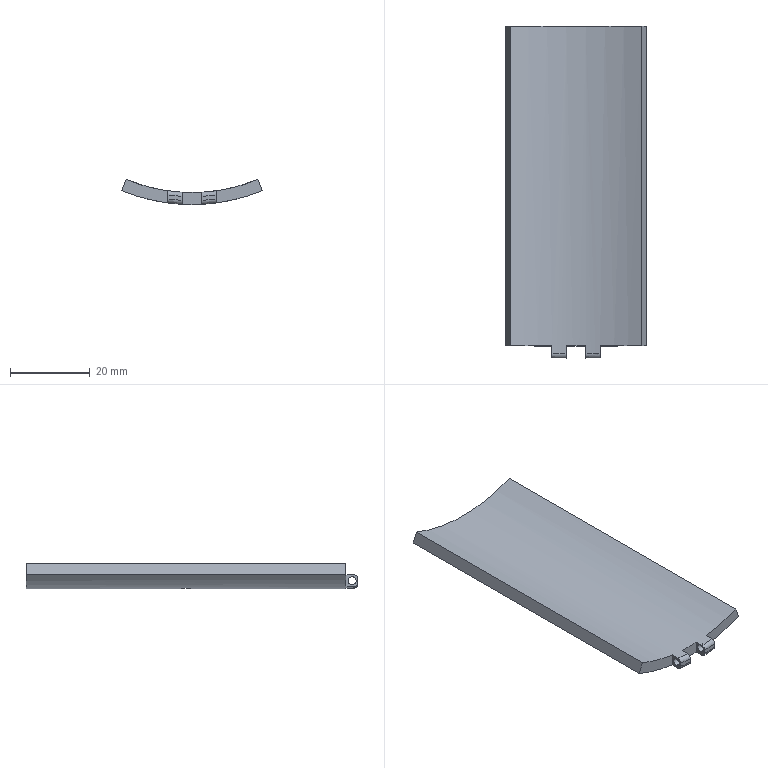Part | SolidWorks | features ICE 3, Blend 1, Fillet 1 | 1 solid | 26 faces | box 35.207 x 83 x 6.273 mm | volume 8409 mm3 | plane 13 | cylinder 9 | torus 4 | commonest cylinder face diameters 2 x4 3 x2 92 x2 86 x1
STEP:
#1=CARTESIAN_POINT('',(-1.5,40.,-45.976));
#2=VERTEX_POINT('',#1);
#3=CARTESIAN_POINT('',(0.,38.5,-46.));
#4=VERTEX_POINT('',#3);
#5=CARTESIAN_POINT('',(-1.5,40.,-45.976));
#6=CARTESIAN_POINT('',(-1.5,39.804,-45.976));
#7=CARTESIAN_POINT('',(-1.461,39.607,-45.977));
#8=CARTESIAN_POINT('',(-1.311,39.246,-45.981));
#9=CARTESIAN_POINT('',(-1.199,39.078,-45.985));
#10=CARTESIAN_POINT('',(-0.9918,38.87,-45.989));
#11=CARTESIAN_POINT('',(-0.9147,38.807,-45.991));
#12=CARTESIAN_POINT('',(-0.7514,38.698,-45.994));
#13=CARTESIAN_POINT('',(-0.6652,38.652,-45.995));
#14=CARTESIAN_POINT('',(-0.4837,38.577,-45.998));
#15=CARTESIAN_POINT('',(-0.3883,38.548,-45.998));
#16=CARTESIAN_POINT('',(-0.1964,38.51,-46.));
#17=CARTESIAN_POINT('',(-0.09898,38.5,-46.));
#18=CARTESIAN_POINT('',(0.,38.5,-46.));
#19=B_SPLINE_CURVE_WITH_KNOTS('',3,(#5,#6,#7,#8,#9,#10,#11,#12,#13,#14,#15,#16,#17,#18),.UNSPECIFIED.,.F.,.F.,(4,2,2,2,2,2,4),(0.00469,0.005276,0.005863,0.006156,0.006449,0.006742,0.007036),.UNSPECIFIED.);
#20=EDGE_CURVE('',#2,#4,#19,.T.);
#21=ORIENTED_EDGE('',*,*,#20,.F.);
#22=CARTESIAN_POINT('',(-1.5,40.,-43.5));
#23=VERTEX_POINT('',#22);
#24=CARTESIAN_POINT('',(-1.5,40.,-46.));
#25=DIRECTION('',(0.,0.,1.));
#26=VECTOR('',#25,1000.);
#27=LINE('',#24,#26);
#28=EDGE_CURVE('',#2,#23,#27,.T.);
#29=ORIENTED_EDGE('',*,*,#28,.T.);
#30=CARTESIAN_POINT('',(1.5,40.,-43.5));
#31=VERTEX_POINT('',#30);
#32=CARTESIAN_POINT('',(0.,40.,-43.5));
#33=DIRECTION('',(0.,0.,1.));
#34=DIRECTION('',(1.,0.,0.));
#35=AXIS2_PLACEMENT_3D('',#32,#33,#34);
#36=CIRCLE('',#35,1.5);
#37=EDGE_CURVE('',#23,#31,#36,.T.);
#38=ORIENTED_EDGE('',*,*,#37,.T.);
#39=CARTESIAN_POINT('',(1.5,40.,-45.976));
#40=VERTEX_POINT('',#39);
#41=CARTESIAN_POINT('',(1.5,40.,-46.));
#42=DIRECTION('',(0.,0.,1.));
#43=VECTOR('',#42,1000.);
#44=LINE('',#41,#43);
#45=EDGE_CURVE('',#40,#31,#44,.T.);
#46=ORIENTED_EDGE('',*,*,#45,.F.);
#47=CARTESIAN_POINT('',(0.,38.5,-46.));
#48=CARTESIAN_POINT('',(0.1978,38.5,-46.));
#49=CARTESIAN_POINT('',(0.3923,38.539,-45.999));
#50=CARTESIAN_POINT('',(0.665,38.652,-45.995));
#51=CARTESIAN_POINT('',(0.7511,38.698,-45.994));
#52=CARTESIAN_POINT('',(0.9139,38.807,-45.991));
#53=CARTESIAN_POINT('',(0.9911,38.87,-45.989));
#54=CARTESIAN_POINT('',(1.199,39.077,-45.985));
#55=CARTESIAN_POINT('',(1.31,39.244,-45.981));
#56=CARTESIAN_POINT('',(1.46,39.605,-45.977));
#57=CARTESIAN_POINT('',(1.5,39.802,-45.976));
#58=CARTESIAN_POINT('',(1.5,40.,-45.976));
#59=B_SPLINE_CURVE_WITH_KNOTS('',3,(#47,#48,#49,#50,#51,#52,#53,#54,#55,#56,#57,#58),.UNSPECIFIED.,.F.,.F.,(4,2,2,2,2,4),(0.007036,0.007622,0.007914,0.008207,0.008793,0.009379),.UNSPECIFIED.);
#60=EDGE_CURVE('',#4,#40,#59,.T.);
#61=ORIENTED_EDGE('',*,*,#60,.F.);
#62=EDGE_LOOP('',(#21,#29,#38,#46,#61));
#63=FACE_OUTER_BOUND('',#62,.T.);
#64=CARTESIAN_POINT('',(0.,40.,-46.));
#65=DIRECTION('',(0.,0.,1.));
#66=DIRECTION('',(1.,0.,0.));
#67=AXIS2_PLACEMENT_3D('',#64,#65,#66);
#68=CYLINDRICAL_SURFACE('',#67,1.5);
#69=ADVANCED_FACE('',(#63),#68,.F.);
#70=CARTESIAN_POINT('',(-6.009,-1.518,-45.081));
#71=VERTEX_POINT('',#70);
#72=CARTESIAN_POINT('',(-6.009,-1.518,-43.081));
#73=VERTEX_POINT('',#72);
#74=CARTESIAN_POINT('',(-6.009,-1.518,-44.081));
#75=DIRECTION('',(-1.,0.,0.));
#76=DIRECTION('',(0.,0.,1.));
#77=AXIS2_PLACEMENT_3D('',#74,#75,#76);
#78=CIRCLE('',#77,1.);
#79=EDGE_CURVE('',#71,#73,#78,.T.);
#80=ORIENTED_EDGE('',*,*,#79,.T.);
#81=CARTESIAN_POINT('',(-2.5,-1.518,-43.081));
#82=VERTEX_POINT('',#81);
#83=CARTESIAN_POINT('',(-6.5,-1.518,-43.081));
#84=DIRECTION('',(1.,0.,0.));
#85=VECTOR('',#84,1000.);
#86=LINE('',#83,#85);
#87=EDGE_CURVE('',#73,#82,#86,.T.);
#88=ORIENTED_EDGE('',*,*,#87,.T.);
#89=CARTESIAN_POINT('',(-2.5,-1.518,-45.081));
#90=VERTEX_POINT('',#89);
#91=CARTESIAN_POINT('',(-2.5,-1.518,-44.081));
#92=DIRECTION('',(1.,0.,0.));
#93=DIRECTION('',(0.,0.,-1.));
#94=AXIS2_PLACEMENT_3D('',#91,#92,#93);
#95=CIRCLE('',#94,1.);
#96=EDGE_CURVE('',#82,#90,#95,.T.);
#97=ORIENTED_EDGE('',*,*,#96,.T.);
#98=CARTESIAN_POINT('',(-6.5,-1.518,-45.081));
#99=DIRECTION('',(1.,0.,0.));
#100=VECTOR('',#99,1000.);
#101=LINE('',#98,#100);
#102=EDGE_CURVE('',#71,#90,#101,.T.);
#103=ORIENTED_EDGE('',*,*,#102,.F.);
#104=EDGE_LOOP('',(#80,#88,#97,#103));
#105=FACE_OUTER_BOUND('',#104,.T.);
#106=CARTESIAN_POINT('',(-6.5,-1.518,-44.081));
#107=DIRECTION('',(1.,0.,0.));
#108=DIRECTION('',(0.,0.,-1.));
#109=AXIS2_PLACEMENT_3D('',#106,#107,#108);
#110=CYLINDRICAL_SURFACE('',#109,1.);
#111=ADVANCED_FACE('',(#105),#110,.F.);
#112=CARTESIAN_POINT('',(2.5,-1.518,-43.081));
#113=VERTEX_POINT('',#112);
#114=CARTESIAN_POINT('',(2.5,-1.518,-45.081));
#115=VERTEX_POINT('',#114);
#116=CARTESIAN_POINT('',(2.5,-1.518,-44.081));
#117=DIRECTION('',(1.,0.,0.));
#118=DIRECTION('',(0.,0.,-1.));
#119=AXIS2_PLACEMENT_3D('',#116,#117,#118);
#120=CIRCLE('',#119,1.);
#121=EDGE_CURVE('',#113,#115,#120,.T.);
#122=ORIENTED_EDGE('',*,*,#121,.F.);
#123=CARTESIAN_POINT('',(6.009,-1.518,-43.081));
#124=VERTEX_POINT('',#123);
#125=CARTESIAN_POINT('',(-6.5,-1.518,-43.081));
#126=DIRECTION('',(1.,0.,0.));
#127=VECTOR('',#126,1000.);
#128=LINE('',#125,#127);
#129=EDGE_CURVE('',#113,#124,#128,.T.);
#130=ORIENTED_EDGE('',*,*,#129,.T.);
#131=CARTESIAN_POINT('',(6.009,-1.518,-45.081));
#132=VERTEX_POINT('',#131);
#133=CARTESIAN_POINT('',(6.009,-1.518,-44.081));
#134=DIRECTION('',(1.,0.,0.));
#135=DIRECTION('',(0.,0.,-1.));
#136=AXIS2_PLACEMENT_3D('',#133,#134,#135);
#137=CIRCLE('',#136,1.);
#138=EDGE_CURVE('',#124,#132,#137,.T.);
#139=ORIENTED_EDGE('',*,*,#138,.T.);
#140=CARTESIAN_POINT('',(-6.5,-1.518,-45.081));
#141=DIRECTION('',(1.,0.,0.));
#142=VECTOR('',#141,1000.);
#143=LINE('',#140,#142);
#144=EDGE_CURVE('',#115,#132,#143,.T.);
#145=ORIENTED_EDGE('',*,*,#144,.F.);
#146=EDGE_LOOP('',(#122,#130,#139,#145));
#147=FACE_OUTER_BOUND('',#146,.T.);
#148=CARTESIAN_POINT('',(-6.5,-1.518,-44.081));
#149=DIRECTION('',(1.,0.,0.));
#150=DIRECTION('',(0.,0.,-1.));
#151=AXIS2_PLACEMENT_3D('',#148,#149,#150);
#152=CYLINDRICAL_SURFACE('',#151,1.);
#153=ADVANCED_FACE('',(#147),#152,.F.);
#154=CARTESIAN_POINT('',(0.,80.,-46.));
#155=VERTEX_POINT('',#154);
#156=CARTESIAN_POINT('',(-17.603,80.,-42.498));
#157=VERTEX_POINT('',#156);
#158=CARTESIAN_POINT('',(0.,80.,0.));
#159=DIRECTION('',(0.,1.,0.));
#160=DIRECTION('',(0.,0.,-1.));
#161=AXIS2_PLACEMENT_3D('',#158,#159,#160);
#162=CIRCLE('',#161,46.);
#163=EDGE_CURVE('',#155,#157,#162,.T.);
#164=ORIENTED_EDGE('',*,*,#163,.F.);
#165=CARTESIAN_POINT('',(0.,41.5,-46.));
#166=VERTEX_POINT('',#165);
#167=CARTESIAN_POINT('',(0.,80.,-46.));
#168=DIRECTION('',(0.,-1.,0.));
#169=VECTOR('',#168,1000.);
#170=LINE('',#167,#169);
#171=EDGE_CURVE('',#155,#166,#170,.T.);
#172=ORIENTED_EDGE('',*,*,#171,.T.);
#173=CARTESIAN_POINT('',(0.,41.5,-46.));
#174=CARTESIAN_POINT('',(-0.09782,41.5,-46.));
#175=CARTESIAN_POINT('',(-0.1972,41.49,-46.));
#176=CARTESIAN_POINT('',(-0.3895,41.452,-45.998));
#177=CARTESIAN_POINT('',(-0.483,41.424,-45.998));
#178=CARTESIAN_POINT('',(-0.6646,41.348,-45.995));
#179=CARTESIAN_POINT('',(-0.7524,41.301,-45.994));
#180=CARTESIAN_POINT('',(-0.9149,41.193,-45.991));
#181=CARTESIAN_POINT('',(-0.9906,41.131,-45.989));
#182=CARTESIAN_POINT('',(-1.201,40.921,-45.985));
#183=CARTESIAN_POINT('',(-1.311,40.756,-45.981));
#184=CARTESIAN_POINT('',(-1.424,40.483,-45.978));
#185=CARTESIAN_POINT('',(-1.452,40.389,-45.977));
#186=CARTESIAN_POINT('',(-1.49,40.197,-45.976));
#187=CARTESIAN_POINT('',(-1.5,40.098,-45.976));
#188=CARTESIAN_POINT('',(-1.5,40.,-45.976));
#189=B_SPLINE_CURVE_WITH_KNOTS('',3,(#173,#174,#175,#176,#177,#178,#179,#180,#181,#182,#183,#184,#185,#186,#187,#188),.UNSPECIFIED.,.F.,.F.,(4,2,2,2,2,2,2,4),(0.002346,0.002639,0.002932,0.003225,0.003518,0.004104,0.004397,0.00469),.UNSPECIFIED.);
#190=EDGE_CURVE('',#166,#2,#189,.T.);
#191=ORIENTED_EDGE('',*,*,#190,.T.);
#192=ORIENTED_EDGE('',*,*,#20,.T.);
#193=CARTESIAN_POINT('',(0.,0.,-46.));
#194=VERTEX_POINT('',#193);
#195=CARTESIAN_POINT('',(0.,80.,-46.));
#196=DIRECTION('',(0.,-1.,0.));
#197=VECTOR('',#196,1000.);
#198=LINE('',#195,#197);
#199=EDGE_CURVE('',#4,#194,#198,.T.);
#200=ORIENTED_EDGE('',*,*,#199,.T.);
#201=CARTESIAN_POINT('',(-2.5,0.,-45.932));
#202=VERTEX_POINT('',#201);
#203=CARTESIAN_POINT('',(0.,0.,0.));
#204=DIRECTION('',(0.,1.,0.));
#205=DIRECTION('',(0.,0.,-1.));
#206=AXIS2_PLACEMENT_3D('',#203,#204,#205);
#207=CIRCLE('',#206,46.);
#208=EDGE_CURVE('',#194,#202,#207,.T.);
#209=ORIENTED_EDGE('',*,*,#208,.T.);
#210=CARTESIAN_POINT('',(-2.5,-2.,-45.932));
#211=VERTEX_POINT('',#210);
#212=CARTESIAN_POINT('',(-2.5,-3.,-45.932));
#213=DIRECTION('',(0.,1.,0.));
#214=VECTOR('',#213,1000.);
#215=LINE('',#212,#214);
#216=EDGE_CURVE('',#211,#202,#215,.T.);
#217=ORIENTED_EDGE('',*,*,#216,.F.);
#218=CARTESIAN_POINT('',(-6.009,-2.,-45.606));
#219=VERTEX_POINT('',#218);
#220=CARTESIAN_POINT('',(0.,-2.,0.));
#221=DIRECTION('',(0.,1.,0.));
#222=DIRECTION('',(0.,0.,-1.));
#223=AXIS2_PLACEMENT_3D('',#220,#221,#222);
#224=CIRCLE('',#223,46.);
#225=EDGE_CURVE('',#211,#219,#224,.T.);
#226=ORIENTED_EDGE('',*,*,#225,.T.);
#227=CARTESIAN_POINT('',(-6.009,0.,-45.606));
#228=VERTEX_POINT('',#227);
#229=CARTESIAN_POINT('',(-6.009,-3.,-45.606));
#230=DIRECTION('',(0.,1.,0.));
#231=VECTOR('',#230,1000.);
#232=LINE('',#229,#231);
#233=EDGE_CURVE('',#219,#228,#232,.T.);
#234=ORIENTED_EDGE('',*,*,#233,.T.);
#235=CARTESIAN_POINT('',(-17.603,0.,-42.498));
#236=VERTEX_POINT('',#235);
#237=CARTESIAN_POINT('',(0.,0.,0.));
#238=DIRECTION('',(0.,1.,0.));
#239=DIRECTION('',(0.,0.,-1.));
#240=AXIS2_PLACEMENT_3D('',#237,#238,#239);
#241=CIRCLE('',#240,46.);
#242=EDGE_CURVE('',#228,#236,#241,.T.);
#243=ORIENTED_EDGE('',*,*,#242,.T.);
#244=CARTESIAN_POINT('',(-17.603,80.,-42.498));
#245=DIRECTION('',(0.,-1.,0.));
#246=VECTOR('',#245,1000.);
#247=LINE('',#244,#246);
#248=EDGE_CURVE('',#157,#236,#247,.T.);
#249=ORIENTED_EDGE('',*,*,#248,.F.);
#250=EDGE_LOOP('',(#164,#172,#191,#192,#200,#209,#217,#226,#234,#243,#249));
#251=FACE_OUTER_BOUND('',#250,.T.);
#252=CARTESIAN_POINT('',(0.,80.,0.));
#253=DIRECTION('',(0.,-1.,0.));
#254=DIRECTION('',(0.,0.,-1.));
#255=AXIS2_PLACEMENT_3D('',#252,#253,#254);
#256=CYLINDRICAL_SURFACE('',#255,46.);
#257=ADVANCED_FACE('',(#251),#256,.T.);
#258=CARTESIAN_POINT('',(2.5,0.,-45.932));
#259=VERTEX_POINT('',#258);
#260=CARTESIAN_POINT('',(0.,0.,0.));
#261=DIRECTION('',(0.,1.,0.));
#262=DIRECTION('',(0.,0.,-1.));
#263=AXIS2_PLACEMENT_3D('',#260,#261,#262);
#264=CIRCLE('',#263,46.);
#265=EDGE_CURVE('',#259,#194,#264,.T.);
#266=ORIENTED_EDGE('',*,*,#265,.F.);
#267=CARTESIAN_POINT('',(2.5,0.,-42.927));
#268=VERTEX_POINT('',#267);
#269=CARTESIAN_POINT('',(2.5,0.,0.));
#270=DIRECTION('',(0.,0.,-1.));
#271=VECTOR('',#270,1000.);
#272=LINE('',#269,#271);
#273=EDGE_CURVE('',#268,#259,#272,.T.);
#274=ORIENTED_EDGE('',*,*,#273,.F.);
#275=CARTESIAN_POINT('',(-2.5,0.,-42.927));
#276=VERTEX_POINT('',#275);
#277=CARTESIAN_POINT('',(0.,0.,0.));
#278=DIRECTION('',(0.,-1.,0.));
#279=DIRECTION('',(0.,0.,-1.));
#280=AXIS2_PLACEMENT_3D('',#277,#278,#279);
#281=CIRCLE('',#280,43.);
#282=EDGE_CURVE('',#276,#268,#281,.T.);
#283=ORIENTED_EDGE('',*,*,#282,.F.);
#284=CARTESIAN_POINT('',(-2.5,0.,0.));
#285=DIRECTION('',(0.,0.,-1.));
#286=VECTOR('',#285,1000.);
#287=LINE('',#284,#286);
#288=EDGE_CURVE('',#276,#202,#287,.T.);
#289=ORIENTED_EDGE('',*,*,#288,.T.);
#290=ORIENTED_EDGE('',*,*,#208,.F.);
#291=EDGE_LOOP('',(#266,#274,#283,#289,#290));
#292=FACE_OUTER_BOUND('',#291,.T.);
#293=CARTESIAN_POINT('',(0.,0.,0.));
#294=DIRECTION('',(0.,-1.,0.));
#295=DIRECTION('',(0.,0.,-1.));
#296=AXIS2_PLACEMENT_3D('',#293,#294,#295);
#297=PLANE('',#296);
#298=ADVANCED_FACE('',(#292),#297,.T.);
#299=ORIENTED_EDGE('',*,*,#242,.F.);
#300=CARTESIAN_POINT('',(-6.009,0.,-42.578));
#301=VERTEX_POINT('',#300);
#302=CARTESIAN_POINT('',(-6.009,0.,0.));
#303=DIRECTION('',(0.,0.,1.));
#304=VECTOR('',#303,1000.);
#305=LINE('',#302,#304);
#306=EDGE_CURVE('',#228,#301,#305,.T.);
#307=ORIENTED_EDGE('',*,*,#306,.T.);
#308=CARTESIAN_POINT('',(-16.455,0.,-39.727));
#309=VERTEX_POINT('',#308);
#310=CARTESIAN_POINT('',(0.,0.,0.));
#311=DIRECTION('',(0.,-1.,0.));
#312=DIRECTION('',(0.,0.,-1.));
#313=AXIS2_PLACEMENT_3D('',#310,#311,#312);
#314=CIRCLE('',#313,43.);
#315=EDGE_CURVE('',#309,#301,#314,.T.);
#316=ORIENTED_EDGE('',*,*,#315,.F.);
#317=CARTESIAN_POINT('',(-17.603,0.,-42.498));
#318=DIRECTION('',(0.3827,0.,0.9239));
#319=VECTOR('',#318,1000.);
#320=LINE('',#317,#319);
#321=EDGE_CURVE('',#236,#309,#320,.T.);
#322=ORIENTED_EDGE('',*,*,#321,.F.);
#323=EDGE_LOOP('',(#299,#307,#316,#322));
#324=FACE_OUTER_BOUND('',#323,.T.);
#325=CARTESIAN_POINT('',(0.,0.,0.));
#326=DIRECTION('',(0.,-1.,0.));
#327=DIRECTION('',(0.,0.,-1.));
#328=AXIS2_PLACEMENT_3D('',#325,#326,#327);
#329=PLANE('',#328);
#330=ADVANCED_FACE('',(#324),#329,.T.);
#331=CARTESIAN_POINT('',(6.009,0.,-42.578));
#332=VERTEX_POINT('',#331);
#333=CARTESIAN_POINT('',(6.009,0.,-45.606));
#334=VERTEX_POINT('',#333);
#335=CARTESIAN_POINT('',(6.009,0.,0.));
#336=DIRECTION('',(0.,0.,-1.));
#337=VECTOR('',#336,1000.);
#338=LINE('',#335,#337);
#339=EDGE_CURVE('',#332,#334,#338,.T.);
#340=ORIENTED_EDGE('',*,*,#339,.T.);
#341=CARTESIAN_POINT('',(17.603,0.,-42.498));
#342=VERTEX_POINT('',#341);
#343=CARTESIAN_POINT('',(0.,0.,0.));
#344=DIRECTION('',(0.,1.,0.));
#345=DIRECTION('',(0.,0.,-1.));
#346=AXIS2_PLACEMENT_3D('',#343,#344,#345);
#347=CIRCLE('',#346,46.);
#348=EDGE_CURVE('',#342,#334,#347,.T.);
#349=ORIENTED_EDGE('',*,*,#348,.F.);
#350=CARTESIAN_POINT('',(16.455,0.,-39.727));
#351=VERTEX_POINT('',#350);
#352=CARTESIAN_POINT('',(17.603,0.,-42.498));
#353=DIRECTION('',(0.3827,0.,-0.9239));
#354=VECTOR('',#353,1000.);
#355=LINE('',#352,#354);
#356=EDGE_CURVE('',#351,#342,#355,.T.);
#357=ORIENTED_EDGE('',*,*,#356,.F.);
#358=CARTESIAN_POINT('',(0.,0.,0.));
#359=DIRECTION('',(0.,-1.,0.));
#360=DIRECTION('',(0.,0.,-1.));
#361=AXIS2_PLACEMENT_3D('',#358,#359,#360);
#362=CIRCLE('',#361,43.);
#363=EDGE_CURVE('',#332,#351,#362,.T.);
#364=ORIENTED_EDGE('',*,*,#363,.F.);
#365=EDGE_LOOP('',(#340,#349,#357,#364));
#366=FACE_OUTER_BOUND('',#365,.T.);
#367=CARTESIAN_POINT('',(0.,0.,0.));
#368=DIRECTION('',(0.,-1.,0.));
#369=DIRECTION('',(0.,0.,-1.));
#370=AXIS2_PLACEMENT_3D('',#367,#368,#369);
#371=PLANE('',#370);
#372=ADVANCED_FACE('',(#366),#371,.T.);
#373=CARTESIAN_POINT('',(-16.455,80.,-39.727));
#374=VERTEX_POINT('',#373);
#375=CARTESIAN_POINT('',(16.455,80.,-39.727));
#376=VERTEX_POINT('',#375);
#377=CARTESIAN_POINT('',(0.,80.,0.));
#378=DIRECTION('',(0.,-1.,0.));
#379=DIRECTION('',(0.,0.,-1.));
#380=AXIS2_PLACEMENT_3D('',#377,#378,#379);
#381=CIRCLE('',#380,43.);
#382=EDGE_CURVE('',#374,#376,#381,.T.);
#383=ORIENTED_EDGE('',*,*,#382,.T.);
#384=CARTESIAN_POINT('',(17.603,80.,-42.498));
#385=VERTEX_POINT('',#384);
#386=CARTESIAN_POINT('',(17.603,80.,-42.498));
#387=DIRECTION('',(0.3827,0.,-0.9239));
#388=VECTOR('',#387,1000.);
#389=LINE('',#386,#388);
#390=EDGE_CURVE('',#376,#385,#389,.T.);
#391=ORIENTED_EDGE('',*,*,#390,.T.);
#392=CARTESIAN_POINT('',(0.,80.,0.));
#393=DIRECTION('',(0.,1.,0.));
#394=DIRECTION('',(0.,0.,-1.));
#395=AXIS2_PLACEMENT_3D('',#392,#393,#394);
#396=CIRCLE('',#395,46.);
#397=EDGE_CURVE('',#385,#155,#396,.T.);
#398=ORIENTED_EDGE('',*,*,#397,.T.);
#399=ORIENTED_EDGE('',*,*,#163,.T.);
#400=CARTESIAN_POINT('',(-17.603,80.,-42.498));
#401=DIRECTION('',(0.3827,0.,0.9239));
#402=VECTOR('',#401,1000.);
#403=LINE('',#400,#402);
#404=EDGE_CURVE('',#157,#374,#403,.T.);
#405=ORIENTED_EDGE('',*,*,#404,.T.);
#406=EDGE_LOOP('',(#383,#391,#398,#399,#405));
#407=FACE_OUTER_BOUND('',#406,.T.);
#408=CARTESIAN_POINT('',(0.,80.,0.));
#409=DIRECTION('',(0.,-1.,0.));
#410=DIRECTION('',(0.,0.,-1.));
#411=AXIS2_PLACEMENT_3D('',#408,#409,#410);
#412=PLANE('',#411);
#413=ADVANCED_FACE('',(#407),#412,.F.);
#414=CARTESIAN_POINT('',(16.455,80.,-39.727));
#415=DIRECTION('',(0.,-1.,0.));
#416=VECTOR('',#415,1000.);
#417=LINE('',#414,#416);
#418=EDGE_CURVE('',#376,#351,#417,.T.);
#419=ORIENTED_EDGE('',*,*,#418,.T.);
#420=ORIENTED_EDGE('',*,*,#356,.T.);
#421=CARTESIAN_POINT('',(17.603,80.,-42.498));
#422=DIRECTION('',(0.,-1.,0.));
#423=VECTOR('',#422,1000.);
#424=LINE('',#421,#423);
#425=EDGE_CURVE('',#385,#342,#424,.T.);
#426=ORIENTED_EDGE('',*,*,#425,.F.);
#427=ORIENTED_EDGE('',*,*,#390,.F.);
#428=EDGE_LOOP('',(#419,#420,#426,#427));
#429=FACE_OUTER_BOUND('',#428,.T.);
#430=CARTESIAN_POINT('',(0.,0.,0.));
#431=DIRECTION('',(0.9239,0.,0.3827));
#432=DIRECTION('',(0.3827,0.,-0.9239));
#433=AXIS2_PLACEMENT_3D('',#430,#431,#432);
#434=PLANE('',#433);
#435=ADVANCED_FACE('',(#429),#434,.T.);
#436=ORIENTED_EDGE('',*,*,#171,.F.);
#437=ORIENTED_EDGE('',*,*,#397,.F.);
#438=ORIENTED_EDGE('',*,*,#425,.T.);
#439=ORIENTED_EDGE('',*,*,#348,.T.);
#440=CARTESIAN_POINT('',(6.009,-2.,-45.606));
#441=VERTEX_POINT('',#440);
#442=CARTESIAN_POINT('',(6.009,-3.,-45.606));
#443=DIRECTION('',(0.,1.,0.));
#444=VECTOR('',#443,1000.);
#445=LINE('',#442,#444);
#446=EDGE_CURVE('',#441,#334,#445,.T.);
#447=ORIENTED_EDGE('',*,*,#446,.F.);
#448=CARTESIAN_POINT('',(2.5,-2.,-45.932));
#449=VERTEX_POINT('',#448);
#450=CARTESIAN_POINT('',(0.,-2.,0.));
#451=DIRECTION('',(0.,1.,0.));
#452=DIRECTION('',(0.,0.,-1.));
#453=AXIS2_PLACEMENT_3D('',#450,#451,#452);
#454=CIRCLE('',#453,46.);
#455=EDGE_CURVE('',#441,#449,#454,.T.);
#456=ORIENTED_EDGE('',*,*,#455,.T.);
#457=CARTESIAN_POINT('',(2.5,-3.,-45.932));
#458=DIRECTION('',(0.,1.,0.));
#459=VECTOR('',#458,1000.);
#460=LINE('',#457,#459);
#461=EDGE_CURVE('',#449,#259,#460,.T.);
#462=ORIENTED_EDGE('',*,*,#461,.T.);
#463=ORIENTED_EDGE('',*,*,#265,.T.);
#464=ORIENTED_EDGE('',*,*,#199,.F.);
#465=ORIENTED_EDGE('',*,*,#60,.T.);
#466=CARTESIAN_POINT('',(1.5,40.,-45.976));
#467=CARTESIAN_POINT('',(1.5,40.099,-45.976));
#468=CARTESIAN_POINT('',(1.49,40.197,-45.976));
#469=CARTESIAN_POINT('',(1.452,40.388,-45.977));
#470=CARTESIAN_POINT('',(1.423,40.484,-45.978));
#471=CARTESIAN_POINT('',(1.348,40.665,-45.98));
#472=CARTESIAN_POINT('',(1.302,40.752,-45.982));
#473=CARTESIAN_POINT('',(1.193,40.915,-45.985));
#474=CARTESIAN_POINT('',(1.13,40.992,-45.986));
#475=CARTESIAN_POINT('',(0.9218,41.199,-45.991));
#476=CARTESIAN_POINT('',(0.7544,41.311,-45.994));
#477=CARTESIAN_POINT('',(0.3932,41.461,-45.999));
#478=CARTESIAN_POINT('',(0.1957,41.5,-46.));
#479=CARTESIAN_POINT('',(0.,41.5,-46.));
#480=B_SPLINE_CURVE_WITH_KNOTS('',3,(#466,#467,#468,#469,#470,#471,#472,#473,#474,#475,#476,#477,#478,#479),.UNSPECIFIED.,.F.,.F.,(4,2,2,2,2,2,4),(0.,0.0002932,0.0005864,0.0008796,0.001173,0.001759,0.002346),.UNSPECIFIED.);
#481=EDGE_CURVE('',#40,#166,#480,.T.);
#482=ORIENTED_EDGE('',*,*,#481,.T.);
#483=EDGE_LOOP('',(#436,#437,#438,#439,#447,#456,#462,#463,#464,#465,#482));
#484=FACE_OUTER_BOUND('',#483,.T.);
#485=CARTESIAN_POINT('',(0.,80.,0.));
#486=DIRECTION('',(0.,-1.,0.));
#487=DIRECTION('',(0.,0.,-1.));
#488=AXIS2_PLACEMENT_3D('',#485,#486,#487);
#489=CYLINDRICAL_SURFACE('',#488,46.);
#490=ADVANCED_FACE('',(#484),#489,.T.);
#491=CARTESIAN_POINT('',(2.5,-2.,-42.927));
#492=VERTEX_POINT('',#491);
#493=CARTESIAN_POINT('',(2.5,-3.,-42.927));
#494=DIRECTION('',(0.,1.,0.));
#495=VECTOR('',#494,1000.);
#496=LINE('',#493,#495);
#497=EDGE_CURVE('',#492,#268,#496,.T.);
#498=ORIENTED_EDGE('',*,*,#497,.F.);
#499=CARTESIAN_POINT('',(6.009,-2.,-42.578));
#500=VERTEX_POINT('',#499);
#501=CARTESIAN_POINT('',(0.,-2.,0.));
#502=DIRECTION('',(0.,-1.,0.));
#503=DIRECTION('',(0.,0.,-1.));
#504=AXIS2_PLACEMENT_3D('',#501,#502,#503);
#505=CIRCLE('',#504,43.);
#506=EDGE_CURVE('',#492,#500,#505,.T.);
#507=ORIENTED_EDGE('',*,*,#506,.T.);
#508=CARTESIAN_POINT('',(6.009,-3.,-42.578));
#509=DIRECTION('',(0.,1.,0.));
#510=VECTOR('',#509,1000.);
#511=LINE('',#508,#510);
#512=EDGE_CURVE('',#500,#332,#511,.T.);
#513=ORIENTED_EDGE('',*,*,#512,.T.);
#514=ORIENTED_EDGE('',*,*,#363,.T.);
#515=ORIENTED_EDGE('',*,*,#418,.F.);
#516=ORIENTED_EDGE('',*,*,#382,.F.);
#517=CARTESIAN_POINT('',(-16.455,80.,-39.727));
#518=DIRECTION('',(0.,-1.,0.));
#519=VECTOR('',#518,1000.);
#520=LINE('',#517,#519);
#521=EDGE_CURVE('',#374,#309,#520,.T.);
#522=ORIENTED_EDGE('',*,*,#521,.T.);
#523=ORIENTED_EDGE('',*,*,#315,.T.);
#524=CARTESIAN_POINT('',(-6.009,-2.,-42.578));
#525=VERTEX_POINT('',#524);
#526=CARTESIAN_POINT('',(-6.009,-3.,-42.578));
#527=DIRECTION('',(0.,1.,0.));
#528=VECTOR('',#527,1000.);
#529=LINE('',#526,#528);
#530=EDGE_CURVE('',#525,#301,#529,.T.);
#531=ORIENTED_EDGE('',*,*,#530,.F.);
#532=CARTESIAN_POINT('',(-2.5,-2.,-42.927));
#533=VERTEX_POINT('',#532);
#534=CARTESIAN_POINT('',(0.,-2.,0.));
#535=DIRECTION('',(0.,-1.,0.));
#536=DIRECTION('',(0.,0.,-1.));
#537=AXIS2_PLACEMENT_3D('',#534,#535,#536);
#538=CIRCLE('',#537,43.);
#539=EDGE_CURVE('',#525,#533,#538,.T.);
#540=ORIENTED_EDGE('',*,*,#539,.T.);
#541=CARTESIAN_POINT('',(-2.5,-3.,-42.927));
#542=DIRECTION('',(0.,1.,0.));
#543=VECTOR('',#542,1000.);
#544=LINE('',#541,#543);
#545=EDGE_CURVE('',#533,#276,#544,.T.);
#546=ORIENTED_EDGE('',*,*,#545,.T.);
#547=ORIENTED_EDGE('',*,*,#282,.T.);
#548=EDGE_LOOP('',(#498,#507,#513,#514,#515,#516,#522,#523,#531,#540,#546,#547));
#549=FACE_OUTER_BOUND('',#548,.T.);
#550=CARTESIAN_POINT('',(0.,80.,0.));
#551=DIRECTION('',(0.,1.,0.));
#552=DIRECTION('',(0.,0.,1.));
#553=AXIS2_PLACEMENT_3D('',#550,#551,#552);
#554=CYLINDRICAL_SURFACE('',#553,43.);
#555=ADVANCED_FACE('',(#549),#554,.F.);
#556=ORIENTED_EDGE('',*,*,#248,.T.);
#557=ORIENTED_EDGE('',*,*,#321,.T.);
#558=ORIENTED_EDGE('',*,*,#521,.F.);
#559=ORIENTED_EDGE('',*,*,#404,.F.);
#560=EDGE_LOOP('',(#556,#557,#558,#559));
#561=FACE_OUTER_BOUND('',#560,.T.);
#562=CARTESIAN_POINT('',(0.,0.,0.));
#563=DIRECTION('',(-0.9239,0.,0.3827));
#564=DIRECTION('',(0.3827,0.,0.9239));
#565=AXIS2_PLACEMENT_3D('',#562,#563,#564);
#566=PLANE('',#565);
#567=ADVANCED_FACE('',(#561),#566,.T.);
#568=ORIENTED_EDGE('',*,*,#79,.F.);
#569=CARTESIAN_POINT('',(-6.009,-1.518,-44.081));
#570=DIRECTION('',(-1.,0.,0.));
#571=DIRECTION('',(0.,0.,1.));
#572=AXIS2_PLACEMENT_3D('',#569,#570,#571);
#573=CIRCLE('',#572,1.);
#574=EDGE_CURVE('',#73,#71,#573,.T.);
#575=ORIENTED_EDGE('',*,*,#574,.F.);
#576=EDGE_LOOP('',(#568,#575));
#577=FACE_BOUND('',#576,.T.);
#578=ORIENTED_EDGE('',*,*,#233,.F.);
#579=CARTESIAN_POINT('',(-6.009,-3.,-44.597));
#580=VERTEX_POINT('',#579);
#581=CARTESIAN_POINT('',(-6.009,-2.,-45.606));
#582=CARTESIAN_POINT('',(-6.009,-2.133,-45.606));
#583=CARTESIAN_POINT('',(-6.009,-2.263,-45.579));
#584=CARTESIAN_POINT('',(-6.009,-2.505,-45.478));
#585=CARTESIAN_POINT('',(-6.009,-2.616,-45.402));
#586=CARTESIAN_POINT('',(-6.009,-2.8,-45.216));
#587=CARTESIAN_POINT('',(-6.009,-2.875,-45.103));
#588=CARTESIAN_POINT('',(-6.009,-2.974,-44.861));
#589=CARTESIAN_POINT('',(-6.009,-3.,-44.73));
#590=CARTESIAN_POINT('',(-6.009,-3.,-44.597));
#591=B_SPLINE_CURVE_WITH_KNOTS('',3,(#581,#582,#583,#584,#585,#586,#587,#588,#589,#590),.UNSPECIFIED.,.F.,.F.,(4,2,2,2,4),(0.,0.0003923,0.0007845,0.001177,0.001569),.UNSPECIFIED.);
#592=EDGE_CURVE('',#219,#580,#591,.T.);
#593=ORIENTED_EDGE('',*,*,#592,.T.);
#594=CARTESIAN_POINT('',(-6.009,-3.,-43.588));
#595=VERTEX_POINT('',#594);
#596=CARTESIAN_POINT('',(-6.009,-3.,0.));
#597=DIRECTION('',(0.,0.,1.));
#598=VECTOR('',#597,1000.);
#599=LINE('',#596,#598);
#600=EDGE_CURVE('',#580,#595,#599,.T.);
#601=ORIENTED_EDGE('',*,*,#600,.T.);
#602=CARTESIAN_POINT('',(-6.009,-3.,-43.588));
#603=CARTESIAN_POINT('',(-6.009,-3.,-43.455));
#604=CARTESIAN_POINT('',(-6.009,-2.974,-43.325));
#605=CARTESIAN_POINT('',(-6.009,-2.875,-43.081));
#606=CARTESIAN_POINT('',(-6.009,-2.801,-42.969));
#607=CARTESIAN_POINT('',(-6.009,-2.525,-42.689));
#608=CARTESIAN_POINT('',(-6.009,-2.265,-42.578));
#609=CARTESIAN_POINT('',(-6.009,-2.,-42.578));
#610=B_SPLINE_CURVE_WITH_KNOTS('',3,(#602,#603,#604,#605,#606,#607,#608,#609),.UNSPECIFIED.,.F.,.F.,(4,2,2,4),(0.,0.0003924,0.0007849,0.00157),.UNSPECIFIED.);
#611=EDGE_CURVE('',#595,#525,#610,.T.);
#612=ORIENTED_EDGE('',*,*,#611,.T.);
#613=ORIENTED_EDGE('',*,*,#530,.T.);
#614=ORIENTED_EDGE('',*,*,#306,.F.);
#615=EDGE_LOOP('',(#578,#593,#601,#612,#613,#614));
#616=FACE_OUTER_BOUND('',#615,.T.);
#617=CARTESIAN_POINT('',(-6.009,-3.,0.));
#618=DIRECTION('',(-1.,0.,0.));
#619=DIRECTION('',(0.,0.,1.));
#620=AXIS2_PLACEMENT_3D('',#617,#618,#619);
#621=PLANE('',#620);
#622=ADVANCED_FACE('',(#577,#616),#621,.T.);
#623=CARTESIAN_POINT('',(-2.5,-1.518,-44.081));
#624=DIRECTION('',(1.,0.,0.));
#625=DIRECTION('',(0.,0.,-1.));
#626=AXIS2_PLACEMENT_3D('',#623,#624,#625);
#627=CIRCLE('',#626,1.);
#628=EDGE_CURVE('',#90,#82,#627,.T.);
#629=ORIENTED_EDGE('',*,*,#628,.F.);
#630=ORIENTED_EDGE('',*,*,#96,.F.);
#631=EDGE_LOOP('',(#629,#630));
#632=FACE_BOUND('',#631,.T.);
#633=CARTESIAN_POINT('',(-2.5,-3.,-43.929));
#634=VERTEX_POINT('',#633);
#635=CARTESIAN_POINT('',(-2.5,-3.,-44.931));
#636=VERTEX_POINT('',#635);
#637=CARTESIAN_POINT('',(-2.5,-3.,0.));
#638=DIRECTION('',(0.,0.,-1.));
#639=VECTOR('',#638,1000.);
#640=LINE('',#637,#639);
#641=EDGE_CURVE('',#634,#636,#640,.T.);
#642=ORIENTED_EDGE('',*,*,#641,.T.);
#643=CARTESIAN_POINT('',(-2.5,-3.,-44.931));
#644=CARTESIAN_POINT('',(-2.5,-3.,-45.063));
#645=CARTESIAN_POINT('',(-2.5,-2.974,-45.192));
#646=CARTESIAN_POINT('',(-2.5,-2.874,-45.435));
#647=CARTESIAN_POINT('',(-2.5,-2.8,-45.546));
#648=CARTESIAN_POINT('',(-2.5,-2.523,-45.823));
#649=CARTESIAN_POINT('',(-2.5,-2.264,-45.932));
#650=CARTESIAN_POINT('',(-2.5,-2.,-45.932));
#651=B_SPLINE_CURVE_WITH_KNOTS('',3,(#643,#644,#645,#646,#647,#648,#649,#650),.UNSPECIFIED.,.F.,.F.,(4,2,2,4),(0.,0.0003908,0.0007817,0.001563),.UNSPECIFIED.);
#652=EDGE_CURVE('',#636,#211,#651,.T.);
#653=ORIENTED_EDGE('',*,*,#652,.T.);
#654=ORIENTED_EDGE('',*,*,#216,.T.);
#655=ORIENTED_EDGE('',*,*,#288,.F.);
#656=ORIENTED_EDGE('',*,*,#545,.F.);
#657=CARTESIAN_POINT('',(-2.5,-2.,-42.927));
#658=CARTESIAN_POINT('',(-2.5,-2.132,-42.927));
#659=CARTESIAN_POINT('',(-2.5,-2.262,-42.953));
#660=CARTESIAN_POINT('',(-2.5,-2.504,-43.054));
#661=CARTESIAN_POINT('',(-2.5,-2.615,-43.128));
#662=CARTESIAN_POINT('',(-2.5,-2.892,-43.405));
#663=CARTESIAN_POINT('',(-2.5,-3.,-43.665));
#664=CARTESIAN_POINT('',(-2.5,-3.,-43.929));
#665=B_SPLINE_CURVE_WITH_KNOTS('',3,(#657,#658,#659,#660,#661,#662,#663,#664),.UNSPECIFIED.,.F.,.F.,(4,2,2,4),(0.,0.0003909,0.0007817,0.001563),.UNSPECIFIED.);
#666=EDGE_CURVE('',#533,#634,#665,.T.);
#667=ORIENTED_EDGE('',*,*,#666,.T.);
#668=EDGE_LOOP('',(#642,#653,#654,#655,#656,#667));
#669=FACE_OUTER_BOUND('',#668,.T.);
#670=CARTESIAN_POINT('',(-2.5,-3.,0.));
#671=DIRECTION('',(1.,0.,0.));
#672=DIRECTION('',(0.,0.,-1.));
#673=AXIS2_PLACEMENT_3D('',#670,#671,#672);
#674=PLANE('',#673);
#675=ADVANCED_FACE('',(#632,#669),#674,.T.);
#676=ORIENTED_EDGE('',*,*,#600,.F.);
#677=CARTESIAN_POINT('',(0.,-3.,0.));
#678=DIRECTION('',(0.,-1.,0.));
#679=DIRECTION('',(0.,0.,-1.));
#680=AXIS2_PLACEMENT_3D('',#677,#678,#679);
#681=CIRCLE('',#680,45.);
#682=EDGE_CURVE('',#580,#636,#681,.T.);
#683=ORIENTED_EDGE('',*,*,#682,.T.);
#684=ORIENTED_EDGE('',*,*,#641,.F.);
#685=CARTESIAN_POINT('',(0.,-3.,0.));
#686=DIRECTION('',(0.,1.,0.));
#687=DIRECTION('',(0.,0.,-1.));
#688=AXIS2_PLACEMENT_3D('',#685,#686,#687);
#689=CIRCLE('',#688,44.);
#690=EDGE_CURVE('',#634,#595,#689,.T.);
#691=ORIENTED_EDGE('',*,*,#690,.T.);
#692=EDGE_LOOP('',(#676,#683,#684,#691));
#693=FACE_OUTER_BOUND('',#692,.T.);
#694=CARTESIAN_POINT('',(0.,-3.,0.));
#695=DIRECTION('',(0.,-1.,0.));
#696=DIRECTION('',(0.,0.,-1.));
#697=AXIS2_PLACEMENT_3D('',#694,#695,#696);
#698=PLANE('',#697);
#699=ADVANCED_FACE('',(#693),#698,.T.);
#700=CARTESIAN_POINT('',(6.009,-1.518,-44.081));
#701=DIRECTION('',(1.,0.,0.));
#702=DIRECTION('',(0.,0.,-1.));
#703=AXIS2_PLACEMENT_3D('',#700,#701,#702);
#704=CIRCLE('',#703,1.);
#705=EDGE_CURVE('',#132,#124,#704,.T.);
#706=ORIENTED_EDGE('',*,*,#705,.F.);
#707=ORIENTED_EDGE('',*,*,#138,.F.);
#708=EDGE_LOOP('',(#706,#707));
#709=FACE_BOUND('',#708,.T.);
#710=CARTESIAN_POINT('',(6.009,-3.,-43.588));
#711=VERTEX_POINT('',#710);
#712=CARTESIAN_POINT('',(6.009,-3.,-44.597));
#713=VERTEX_POINT('',#712);
#714=CARTESIAN_POINT('',(6.009,-3.,0.));
#715=DIRECTION('',(0.,0.,-1.));
#716=VECTOR('',#715,1000.);
#717=LINE('',#714,#716);
#718=EDGE_CURVE('',#711,#713,#717,.T.);
#719=ORIENTED_EDGE('',*,*,#718,.T.);
#720=CARTESIAN_POINT('',(6.009,-3.,-44.597));
#721=CARTESIAN_POINT('',(6.009,-3.,-44.73));
#722=CARTESIAN_POINT('',(6.009,-2.974,-44.86));
#723=CARTESIAN_POINT('',(6.009,-2.875,-45.103));
#724=CARTESIAN_POINT('',(6.009,-2.801,-45.215));
#725=CARTESIAN_POINT('',(6.009,-2.525,-45.495));
#726=CARTESIAN_POINT('',(6.009,-2.265,-45.606));
#727=CARTESIAN_POINT('',(6.009,-2.,-45.606));
#728=B_SPLINE_CURVE_WITH_KNOTS('',3,(#720,#721,#722,#723,#724,#725,#726,#727),.UNSPECIFIED.,.F.,.F.,(4,2,2,4),(0.,0.0003923,0.0007846,0.001569),.UNSPECIFIED.);
#729=EDGE_CURVE('',#713,#441,#728,.T.);
#730=ORIENTED_EDGE('',*,*,#729,.T.);
#731=ORIENTED_EDGE('',*,*,#446,.T.);
#732=ORIENTED_EDGE('',*,*,#339,.F.);
#733=ORIENTED_EDGE('',*,*,#512,.F.);
#734=CARTESIAN_POINT('',(6.009,-2.,-42.578));
#735=CARTESIAN_POINT('',(6.009,-2.133,-42.578));
#736=CARTESIAN_POINT('',(6.009,-2.263,-42.605));
#737=CARTESIAN_POINT('',(6.009,-2.506,-42.707));
#738=CARTESIAN_POINT('',(6.009,-2.617,-42.782));
#739=CARTESIAN_POINT('',(6.009,-2.801,-42.969));
#740=CARTESIAN_POINT('',(6.009,-2.875,-43.081));
#741=CARTESIAN_POINT('',(6.009,-2.974,-43.323));
#742=CARTESIAN_POINT('',(6.009,-3.,-43.455));
#743=CARTESIAN_POINT('',(6.009,-3.,-43.588));
#744=B_SPLINE_CURVE_WITH_KNOTS('',3,(#734,#735,#736,#737,#738,#739,#740,#741,#742,#743),.UNSPECIFIED.,.F.,.F.,(4,2,2,2,4),(0.,0.0003924,0.0007849,0.001177,0.00157),.UNSPECIFIED.);
#745=EDGE_CURVE('',#500,#711,#744,.T.);
#746=ORIENTED_EDGE('',*,*,#745,.T.);
#747=EDGE_LOOP('',(#719,#730,#731,#732,#733,#746));
#748=FACE_OUTER_BOUND('',#747,.T.);
#749=CARTESIAN_POINT('',(6.009,-3.,0.));
#750=DIRECTION('',(1.,0.,0.));
#751=DIRECTION('',(0.,0.,-1.));
#752=AXIS2_PLACEMENT_3D('',#749,#750,#751);
#753=PLANE('',#752);
#754=ADVANCED_FACE('',(#709,#748),#753,.T.);
#755=CARTESIAN_POINT('',(2.5,-1.518,-44.081));
#756=DIRECTION('',(1.,0.,0.));
#757=DIRECTION('',(0.,0.,-1.));
#758=AXIS2_PLACEMENT_3D('',#755,#756,#757);
#759=CIRCLE('',#758,1.);
#760=EDGE_CURVE('',#115,#113,#759,.T.);
#761=ORIENTED_EDGE('',*,*,#760,.T.);
#762=ORIENTED_EDGE('',*,*,#121,.T.);
#763=EDGE_LOOP('',(#761,#762));
#764=FACE_BOUND('',#763,.T.);
#765=ORIENTED_EDGE('',*,*,#461,.F.);
#766=CARTESIAN_POINT('',(2.5,-3.,-44.931));
#767=VERTEX_POINT('',#766);
#768=CARTESIAN_POINT('',(2.5,-2.,-45.932));
#769=CARTESIAN_POINT('',(2.5,-2.132,-45.932));
#770=CARTESIAN_POINT('',(2.5,-2.262,-45.906));
#771=CARTESIAN_POINT('',(2.5,-2.504,-45.805));
#772=CARTESIAN_POINT('',(2.5,-2.615,-45.731));
#773=CARTESIAN_POINT('',(2.5,-2.892,-45.454));
#774=CARTESIAN_POINT('',(2.5,-3.,-45.195));
#775=CARTESIAN_POINT('',(2.5,-3.,-44.931));
#776=B_SPLINE_CURVE_WITH_KNOTS('',3,(#768,#769,#770,#771,#772,#773,#774,#775),.UNSPECIFIED.,.F.,.F.,(4,2,2,4),(0.,0.0003908,0.0007817,0.001563),.UNSPECIFIED.);
#777=EDGE_CURVE('',#449,#767,#776,.T.);
#778=ORIENTED_EDGE('',*,*,#777,.T.);
#779=CARTESIAN_POINT('',(2.5,-3.,-43.929));
#780=VERTEX_POINT('',#779);
#781=CARTESIAN_POINT('',(2.5,-3.,0.));
#782=DIRECTION('',(0.,0.,-1.));
#783=VECTOR('',#782,1000.);
#784=LINE('',#781,#783);
#785=EDGE_CURVE('',#780,#767,#784,.T.);
#786=ORIENTED_EDGE('',*,*,#785,.F.);
#787=CARTESIAN_POINT('',(2.5,-3.,-43.929));
#788=CARTESIAN_POINT('',(2.5,-3.,-43.797));
#789=CARTESIAN_POINT('',(2.5,-2.974,-43.667));
#790=CARTESIAN_POINT('',(2.5,-2.874,-43.425));
#791=CARTESIAN_POINT('',(2.5,-2.8,-43.314));
#792=CARTESIAN_POINT('',(2.5,-2.523,-43.036));
#793=CARTESIAN_POINT('',(2.5,-2.264,-42.927));
#794=CARTESIAN_POINT('',(2.5,-2.,-42.927));
#795=B_SPLINE_CURVE_WITH_KNOTS('',3,(#787,#788,#789,#790,#791,#792,#793,#794),.UNSPECIFIED.,.F.,.F.,(4,2,2,4),(0.,0.0003909,0.0007817,0.001563),.UNSPECIFIED.);
#796=EDGE_CURVE('',#780,#492,#795,.T.);
#797=ORIENTED_EDGE('',*,*,#796,.T.);
#798=ORIENTED_EDGE('',*,*,#497,.T.);
#799=ORIENTED_EDGE('',*,*,#273,.T.);
#800=EDGE_LOOP('',(#765,#778,#786,#797,#798,#799));
#801=FACE_OUTER_BOUND('',#800,.T.);
#802=CARTESIAN_POINT('',(2.5,-3.,0.));
#803=DIRECTION('',(1.,0.,0.));
#804=DIRECTION('',(0.,0.,-1.));
#805=AXIS2_PLACEMENT_3D('',#802,#803,#804);
#806=PLANE('',#805);
#807=ADVANCED_FACE('',(#764,#801),#806,.F.);
#808=ORIENTED_EDGE('',*,*,#785,.T.);
#809=CARTESIAN_POINT('',(0.,-3.,0.));
#810=DIRECTION('',(0.,-1.,0.));
#811=DIRECTION('',(0.,0.,-1.));
#812=AXIS2_PLACEMENT_3D('',#809,#810,#811);
#813=CIRCLE('',#812,45.);
#814=EDGE_CURVE('',#767,#713,#813,.T.);
#815=ORIENTED_EDGE('',*,*,#814,.T.);
#816=ORIENTED_EDGE('',*,*,#718,.F.);
#817=CARTESIAN_POINT('',(0.,-3.,0.));
#818=DIRECTION('',(0.,1.,0.));
#819=DIRECTION('',(0.,0.,-1.));
#820=AXIS2_PLACEMENT_3D('',#817,#818,#819);
#821=CIRCLE('',#820,44.);
#822=EDGE_CURVE('',#711,#780,#821,.T.);
#823=ORIENTED_EDGE('',*,*,#822,.T.);
#824=EDGE_LOOP('',(#808,#815,#816,#823));
#825=FACE_OUTER_BOUND('',#824,.T.);
#826=CARTESIAN_POINT('',(0.,-3.,0.));
#827=DIRECTION('',(0.,-1.,0.));
#828=DIRECTION('',(0.,0.,-1.));
#829=AXIS2_PLACEMENT_3D('',#826,#827,#828);
#830=PLANE('',#829);
#831=ADVANCED_FACE('',(#825),#830,.T.);
#832=ORIENTED_EDGE('',*,*,#129,.F.);
#833=ORIENTED_EDGE('',*,*,#760,.F.);
#834=ORIENTED_EDGE('',*,*,#144,.T.);
#835=ORIENTED_EDGE('',*,*,#705,.T.);
#836=EDGE_LOOP('',(#832,#833,#834,#835));
#837=FACE_OUTER_BOUND('',#836,.T.);
#838=CARTESIAN_POINT('',(-6.5,-1.518,-44.081));
#839=DIRECTION('',(1.,0.,0.));
#840=DIRECTION('',(0.,0.,-1.));
#841=AXIS2_PLACEMENT_3D('',#838,#839,#840);
#842=CYLINDRICAL_SURFACE('',#841,1.);
#843=ADVANCED_FACE('',(#837),#842,.F.);
#844=ORIENTED_EDGE('',*,*,#87,.F.);
#845=ORIENTED_EDGE('',*,*,#574,.T.);
#846=ORIENTED_EDGE('',*,*,#102,.T.);
#847=ORIENTED_EDGE('',*,*,#628,.T.);
#848=EDGE_LOOP('',(#844,#845,#846,#847));
#849=FACE_OUTER_BOUND('',#848,.T.);
#850=CARTESIAN_POINT('',(-6.5,-1.518,-44.081));
#851=DIRECTION('',(1.,0.,0.));
#852=DIRECTION('',(0.,0.,-1.));
#853=AXIS2_PLACEMENT_3D('',#850,#851,#852);
#854=CYLINDRICAL_SURFACE('',#853,1.);
#855=ADVANCED_FACE('',(#849),#854,.F.);
#856=ORIENTED_EDGE('',*,*,#777,.F.);
#857=ORIENTED_EDGE('',*,*,#455,.F.);
#858=ORIENTED_EDGE('',*,*,#729,.F.);
#859=ORIENTED_EDGE('',*,*,#814,.F.);
#860=EDGE_LOOP('',(#856,#857,#858,#859));
#861=FACE_OUTER_BOUND('',#860,.T.);
#862=CARTESIAN_POINT('',(0.,-2.,0.));
#863=DIRECTION('',(0.,-1.,0.));
#864=DIRECTION('',(0.,0.,-1.));
#865=AXIS2_PLACEMENT_3D('',#862,#863,#864);
#866=TOROIDAL_SURFACE('',#865,45.,1.);
#867=ADVANCED_FACE('',(#861),#866,.T.);
#868=ORIENTED_EDGE('',*,*,#745,.F.);
#869=ORIENTED_EDGE('',*,*,#506,.F.);
#870=ORIENTED_EDGE('',*,*,#796,.F.);
#871=ORIENTED_EDGE('',*,*,#822,.F.);
#872=EDGE_LOOP('',(#868,#869,#870,#871));
#873=FACE_OUTER_BOUND('',#872,.T.);
#874=CARTESIAN_POINT('',(0.,-2.,0.));
#875=DIRECTION('',(0.,-1.,0.));
#876=DIRECTION('',(0.,0.,-1.));
#877=AXIS2_PLACEMENT_3D('',#874,#875,#876);
#878=TOROIDAL_SURFACE('',#877,44.,1.);
#879=ADVANCED_FACE('',(#873),#878,.T.);
#880=ORIENTED_EDGE('',*,*,#592,.F.);
#881=ORIENTED_EDGE('',*,*,#225,.F.);
#882=ORIENTED_EDGE('',*,*,#652,.F.);
#883=ORIENTED_EDGE('',*,*,#682,.F.);
#884=EDGE_LOOP('',(#880,#881,#882,#883));
#885=FACE_OUTER_BOUND('',#884,.T.);
#886=CARTESIAN_POINT('',(0.,-2.,0.));
#887=DIRECTION('',(0.,-1.,0.));
#888=DIRECTION('',(0.,0.,-1.));
#889=AXIS2_PLACEMENT_3D('',#886,#887,#888);
#890=TOROIDAL_SURFACE('',#889,45.,1.);
#891=ADVANCED_FACE('',(#885),#890,.T.);
#892=ORIENTED_EDGE('',*,*,#666,.F.);
#893=ORIENTED_EDGE('',*,*,#539,.F.);
#894=ORIENTED_EDGE('',*,*,#611,.F.);
#895=ORIENTED_EDGE('',*,*,#690,.F.);
#896=EDGE_LOOP('',(#892,#893,#894,#895));
#897=FACE_OUTER_BOUND('',#896,.T.);
#898=CARTESIAN_POINT('',(0.,-2.,0.));
#899=DIRECTION('',(0.,-1.,0.));
#900=DIRECTION('',(0.,0.,-1.));
#901=AXIS2_PLACEMENT_3D('',#898,#899,#900);
#902=TOROIDAL_SURFACE('',#901,44.,1.);
#903=ADVANCED_FACE('',(#897),#902,.T.);
#904=ORIENTED_EDGE('',*,*,#28,.F.);
#905=ORIENTED_EDGE('',*,*,#190,.F.);
#906=ORIENTED_EDGE('',*,*,#481,.F.);
#907=ORIENTED_EDGE('',*,*,#45,.T.);
#908=CARTESIAN_POINT('',(0.,40.,-43.5));
#909=DIRECTION('',(0.,0.,1.));
#910=DIRECTION('',(1.,0.,0.));
#911=AXIS2_PLACEMENT_3D('',#908,#909,#910);
#912=CIRCLE('',#911,1.5);
#913=EDGE_CURVE('',#31,#23,#912,.T.);
#914=ORIENTED_EDGE('',*,*,#913,.T.);
#915=EDGE_LOOP('',(#904,#905,#906,#907,#914));
#916=FACE_OUTER_BOUND('',#915,.T.);
#917=CARTESIAN_POINT('',(0.,40.,-46.));
#918=DIRECTION('',(0.,0.,1.));
#919=DIRECTION('',(1.,0.,0.));
#920=AXIS2_PLACEMENT_3D('',#917,#918,#919);
#921=CYLINDRICAL_SURFACE('',#920,1.5);
#922=ADVANCED_FACE('',(#916),#921,.F.);
#923=ORIENTED_EDGE('',*,*,#913,.F.);
#924=ORIENTED_EDGE('',*,*,#37,.F.);
#925=EDGE_LOOP('',(#923,#924));
#926=FACE_OUTER_BOUND('',#925,.T.);
#927=CARTESIAN_POINT('',(0.,40.,-43.5));
#928=DIRECTION('',(0.,0.,1.));
#929=DIRECTION('',(1.,0.,0.));
#930=AXIS2_PLACEMENT_3D('',#927,#928,#929);
#931=PLANE('',#930);
#932=ADVANCED_FACE('',(#926),#931,.F.);
#933=CLOSED_SHELL('',(#69,#111,#153,#257,#298,#330,#372,#413,#435,#490,#555,#567,#622,#675,#699,#754,#807,#831,#843,#855,#867,#879,#891,#903,#922,#932));
#934=MANIFOLD_SOLID_BREP('',#933);
#935=CARTESIAN_POINT('',(0.,0.,0.));
#936=DIRECTION('',(0.,0.,1.));
#937=DIRECTION('',(1.,0.,0.));
#938=AXIS2_PLACEMENT_3D('',#935,#936,#937);
#939=(LENGTH_UNIT()NAMED_UNIT(*)SI_UNIT(.MILLI.,.METRE.));
#940=UNCERTAINTY_MEASURE_WITH_UNIT(LENGTH_MEASURE(0.00001),#939,'','');
#941=(NAMED_UNIT(*)PLANE_ANGLE_UNIT()SI_UNIT($,.RADIAN.));
#942=(NAMED_UNIT(*)SI_UNIT($,.STERADIAN.)SOLID_ANGLE_UNIT());
#943=(GEOMETRIC_REPRESENTATION_CONTEXT(3)GLOBAL_UNCERTAINTY_ASSIGNED_CONTEXT((#940))GLOBAL_UNIT_ASSIGNED_CONTEXT((#939,#941,#942))REPRESENTATION_CONTEXT('',''));
#944=ADVANCED_BREP_SHAPE_REPRESENTATION('',(#934,#938),#943);